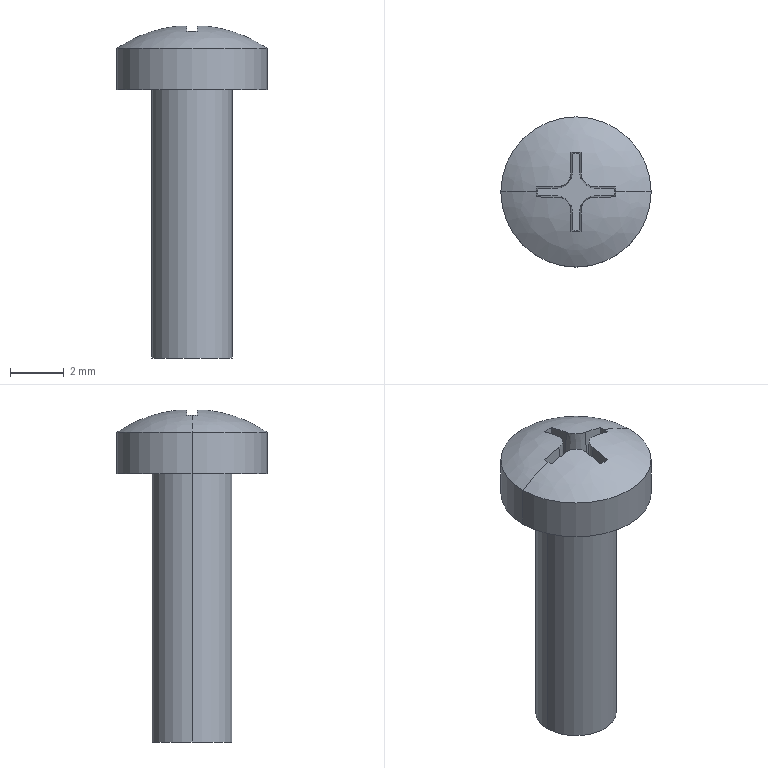Part | STEP file | GB818-M3X10-ZN-4.8_1 | 1 solid | 26 faces | box 5.6 x 5.6 x 12.376 mm | volume 116.575 mm3 | plane 11 | cone 9 | cylinder 4 | spline 2 | commonest cylinder face diameters 3 x2 5.6 x2